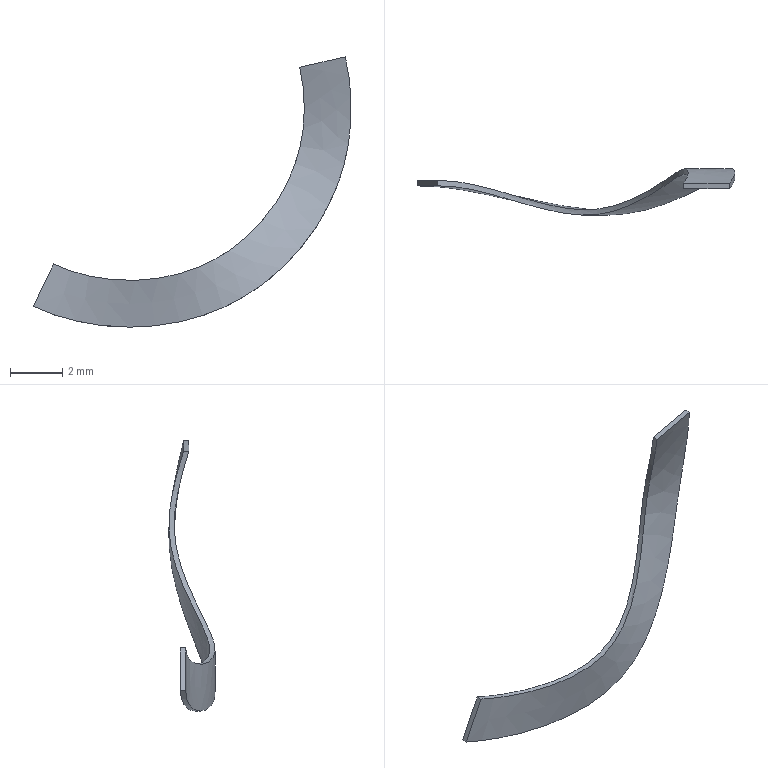Part | NX | features ODD_TURNS_COMBINE 2 | 1 solid | 6 faces | box 12.214 x 1.775 x 10.382 mm | volume 6.257 mm3 | spline 4 | plane 2